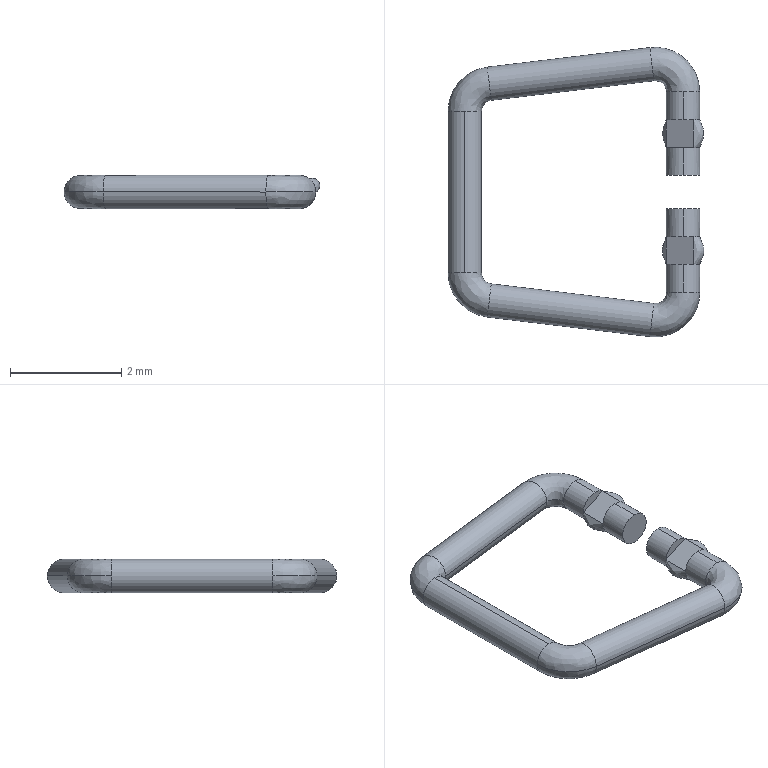Part | SolidWorks | features BaseBody 1, Scale 1 | 1 solid | 40 faces | box 4.596 x 5.2 x 0.6 mm | volume 4.12 mm3 | cylinder 14 | plane 14 | spline 12 | commonest cylinder face diameters 0.6 x14